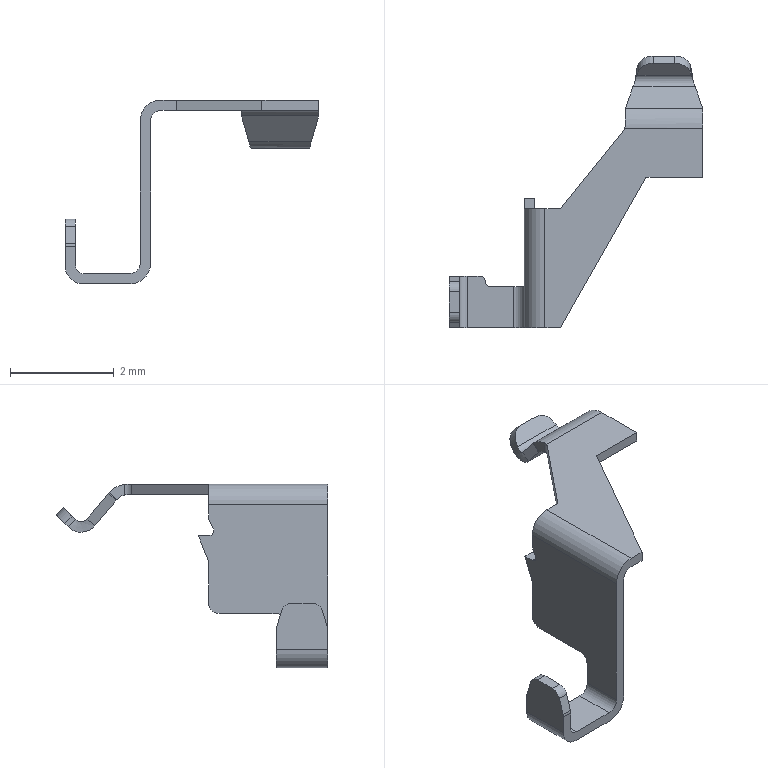Part | Creo | 1 solid | 60 faces | box 4.9 x 5.245 x 3.55 mm | volume 3.146 mm3 | plane 34 | cylinder 22 | spline 4 | commonest cylinder face diameters 0.4 x9 0.2 x3 0.6 x3 0.3 x2 0.7 x2 0.8 x2